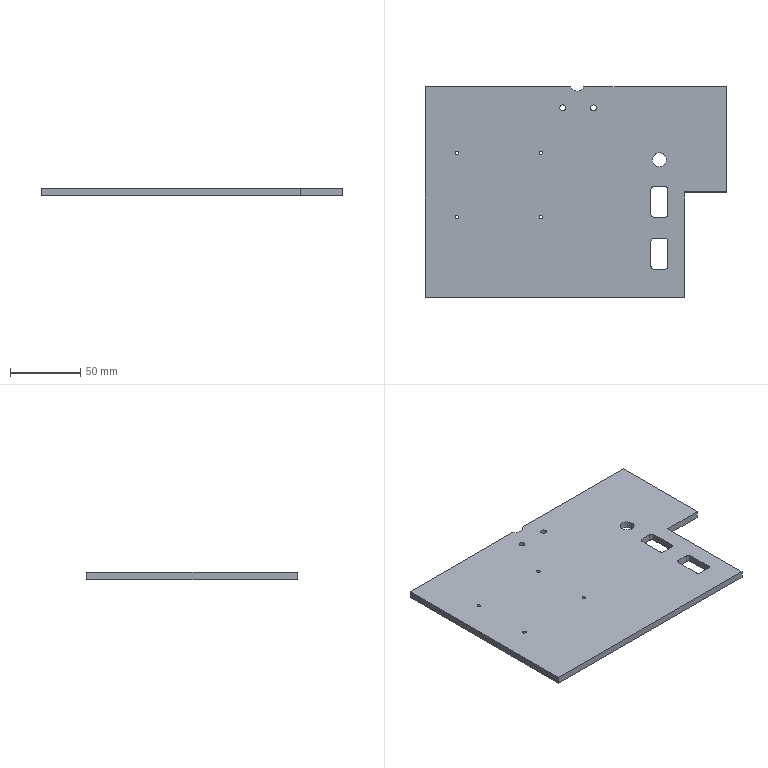Part | NX | features BREP 1 | 1 solid | 33 faces | box 215 x 150 x 5 mm | volume 146666 mm3 | plane 17 | cylinder 16 | commonest cylinder face diameters 4 x8 2.5 x4 4.2 x2 10 x2
STEP:
#1=CARTESIAN_POINT('',(-68.75,28.,0.));
#2=VERTEX_POINT('',#1);
#3=CARTESIAN_POINT('',(-70.,28.,0.));
#4=DIRECTION('',(0.,0.,1.));
#5=DIRECTION('',(1.,0.,0.));
#6=AXIS2_PLACEMENT_3D('',#3,#4,#5);
#7=CIRCLE('',#6,1.25);
#8=EDGE_CURVE('',#2,#2,#7,.T.);
#9=ORIENTED_EDGE('',*,*,#8,.T.);
#10=EDGE_LOOP('',(#9));
#11=FACE_BOUND('',#10,.T.);
#12=CARTESIAN_POINT('',(-71.25,28.,-5.));
#13=VERTEX_POINT('',#12);
#14=CARTESIAN_POINT('',(-70.,28.,-5.));
#15=DIRECTION('',(0.,0.,-1.));
#16=DIRECTION('',(-1.,0.,0.));
#17=AXIS2_PLACEMENT_3D('',#14,#15,#16);
#18=CIRCLE('',#17,1.25);
#19=EDGE_CURVE('',#13,#13,#18,.T.);
#20=ORIENTED_EDGE('',*,*,#19,.T.);
#21=EDGE_LOOP('',(#20));
#22=FACE_BOUND('',#21,.T.);
#23=CARTESIAN_POINT('',(-70.,28.,-10.));
#24=DIRECTION('',(0.,0.,1.));
#25=DIRECTION('',(1.,0.,0.));
#26=AXIS2_PLACEMENT_3D('',#23,#24,#25);
#27=CYLINDRICAL_SURFACE('',#26,1.25);
#28=ADVANCED_FACE('',(#11,#22),#27,.F.);
#29=CARTESIAN_POINT('',(-8.75,-18.,0.));
#30=VERTEX_POINT('',#29);
#31=CARTESIAN_POINT('',(-10.,-18.,0.));
#32=DIRECTION('',(0.,0.,1.));
#33=DIRECTION('',(1.,0.,0.));
#34=AXIS2_PLACEMENT_3D('',#31,#32,#33);
#35=CIRCLE('',#34,1.25);
#36=EDGE_CURVE('',#30,#30,#35,.T.);
#37=ORIENTED_EDGE('',*,*,#36,.T.);
#38=EDGE_LOOP('',(#37));
#39=FACE_BOUND('',#38,.T.);
#40=CARTESIAN_POINT('',(-11.25,-18.,-5.));
#41=VERTEX_POINT('',#40);
#42=CARTESIAN_POINT('',(-10.,-18.,-5.));
#43=DIRECTION('',(0.,0.,-1.));
#44=DIRECTION('',(-1.,0.,0.));
#45=AXIS2_PLACEMENT_3D('',#42,#43,#44);
#46=CIRCLE('',#45,1.25);
#47=EDGE_CURVE('',#41,#41,#46,.T.);
#48=ORIENTED_EDGE('',*,*,#47,.T.);
#49=EDGE_LOOP('',(#48));
#50=FACE_BOUND('',#49,.T.);
#51=CARTESIAN_POINT('',(-10.,-18.,-10.));
#52=DIRECTION('',(0.,0.,1.));
#53=DIRECTION('',(1.,0.,0.));
#54=AXIS2_PLACEMENT_3D('',#51,#52,#53);
#55=CYLINDRICAL_SURFACE('',#54,1.25);
#56=ADVANCED_FACE('',(#39,#50),#55,.F.);
#57=CARTESIAN_POINT('',(-8.75,28.,0.));
#58=VERTEX_POINT('',#57);
#59=CARTESIAN_POINT('',(-10.,28.,0.));
#60=DIRECTION('',(0.,0.,1.));
#61=DIRECTION('',(1.,0.,0.));
#62=AXIS2_PLACEMENT_3D('',#59,#60,#61);
#63=CIRCLE('',#62,1.25);
#64=EDGE_CURVE('',#58,#58,#63,.T.);
#65=ORIENTED_EDGE('',*,*,#64,.T.);
#66=EDGE_LOOP('',(#65));
#67=FACE_BOUND('',#66,.T.);
#68=CARTESIAN_POINT('',(-11.25,28.,-5.));
#69=VERTEX_POINT('',#68);
#70=CARTESIAN_POINT('',(-10.,28.,-5.));
#71=DIRECTION('',(0.,0.,-1.));
#72=DIRECTION('',(-1.,0.,0.));
#73=AXIS2_PLACEMENT_3D('',#70,#71,#72);
#74=CIRCLE('',#73,1.25);
#75=EDGE_CURVE('',#69,#69,#74,.T.);
#76=ORIENTED_EDGE('',*,*,#75,.T.);
#77=EDGE_LOOP('',(#76));
#78=FACE_BOUND('',#77,.T.);
#79=CARTESIAN_POINT('',(-10.,28.,-10.));
#80=DIRECTION('',(0.,0.,1.));
#81=DIRECTION('',(1.,0.,0.));
#82=AXIS2_PLACEMENT_3D('',#79,#80,#81);
#83=CYLINDRICAL_SURFACE('',#82,1.25);
#84=ADVANCED_FACE('',(#67,#78),#83,.F.);
#85=CARTESIAN_POINT('',(-68.75,-18.,0.));
#86=VERTEX_POINT('',#85);
#87=CARTESIAN_POINT('',(-70.,-18.,0.));
#88=DIRECTION('',(0.,0.,1.));
#89=DIRECTION('',(1.,0.,0.));
#90=AXIS2_PLACEMENT_3D('',#87,#88,#89);
#91=CIRCLE('',#90,1.25);
#92=EDGE_CURVE('',#86,#86,#91,.T.);
#93=ORIENTED_EDGE('',*,*,#92,.T.);
#94=EDGE_LOOP('',(#93));
#95=FACE_BOUND('',#94,.T.);
#96=CARTESIAN_POINT('',(-71.25,-18.,-5.));
#97=VERTEX_POINT('',#96);
#98=CARTESIAN_POINT('',(-70.,-18.,-5.));
#99=DIRECTION('',(0.,0.,-1.));
#100=DIRECTION('',(-1.,0.,0.));
#101=AXIS2_PLACEMENT_3D('',#98,#99,#100);
#102=CIRCLE('',#101,1.25);
#103=EDGE_CURVE('',#97,#97,#102,.T.);
#104=ORIENTED_EDGE('',*,*,#103,.T.);
#105=EDGE_LOOP('',(#104));
#106=FACE_BOUND('',#105,.T.);
#107=CARTESIAN_POINT('',(-70.,-18.,-10.));
#108=DIRECTION('',(0.,0.,1.));
#109=DIRECTION('',(1.,0.,0.));
#110=AXIS2_PLACEMENT_3D('',#107,#108,#109);
#111=CYLINDRICAL_SURFACE('',#110,1.25);
#112=ADVANCED_FACE('',(#95,#106),#111,.F.);
#113=CARTESIAN_POINT('',(3.4,60.,-5.));
#114=VERTEX_POINT('',#113);
#115=CARTESIAN_POINT('',(5.5,60.,-5.));
#116=DIRECTION('',(0.,0.,-1.));
#117=DIRECTION('',(-1.,0.,0.));
#118=AXIS2_PLACEMENT_3D('',#115,#116,#117);
#119=CIRCLE('',#118,2.1);
#120=EDGE_CURVE('',#114,#114,#119,.T.);
#121=ORIENTED_EDGE('',*,*,#120,.T.);
#122=EDGE_LOOP('',(#121));
#123=FACE_BOUND('',#122,.T.);
#124=CARTESIAN_POINT('',(3.4,60.,0.));
#125=VERTEX_POINT('',#124);
#126=CARTESIAN_POINT('',(5.5,60.,0.));
#127=DIRECTION('',(0.,0.,-1.));
#128=DIRECTION('',(-1.,0.,0.));
#129=AXIS2_PLACEMENT_3D('',#126,#127,#128);
#130=CIRCLE('',#129,2.1);
#131=EDGE_CURVE('',#125,#125,#130,.T.);
#132=ORIENTED_EDGE('',*,*,#131,.F.);
#133=EDGE_LOOP('',(#132));
#134=FACE_BOUND('',#133,.T.);
#135=CARTESIAN_POINT('',(5.5,60.,-5.));
#136=DIRECTION('',(0.,0.,-1.));
#137=DIRECTION('',(-1.,0.,0.));
#138=AXIS2_PLACEMENT_3D('',#135,#136,#137);
#139=CYLINDRICAL_SURFACE('',#138,2.1);
#140=ADVANCED_FACE('',(#123,#134),#139,.F.);
#141=CARTESIAN_POINT('',(25.4,60.,-5.));
#142=VERTEX_POINT('',#141);
#143=CARTESIAN_POINT('',(27.5,60.,-5.));
#144=DIRECTION('',(0.,0.,-1.));
#145=DIRECTION('',(-1.,0.,0.));
#146=AXIS2_PLACEMENT_3D('',#143,#144,#145);
#147=CIRCLE('',#146,2.1);
#148=EDGE_CURVE('',#142,#142,#147,.T.);
#149=ORIENTED_EDGE('',*,*,#148,.T.);
#150=EDGE_LOOP('',(#149));
#151=FACE_BOUND('',#150,.T.);
#152=CARTESIAN_POINT('',(25.4,60.,0.));
#153=VERTEX_POINT('',#152);
#154=CARTESIAN_POINT('',(27.5,60.,0.));
#155=DIRECTION('',(0.,0.,-1.));
#156=DIRECTION('',(-1.,0.,0.));
#157=AXIS2_PLACEMENT_3D('',#154,#155,#156);
#158=CIRCLE('',#157,2.1);
#159=EDGE_CURVE('',#153,#153,#158,.T.);
#160=ORIENTED_EDGE('',*,*,#159,.F.);
#161=EDGE_LOOP('',(#160));
#162=FACE_BOUND('',#161,.T.);
#163=CARTESIAN_POINT('',(27.5,60.,-5.));
#164=DIRECTION('',(0.,0.,-1.));
#165=DIRECTION('',(-1.,0.,0.));
#166=AXIS2_PLACEMENT_3D('',#163,#164,#165);
#167=CYLINDRICAL_SURFACE('',#166,2.1);
#168=ADVANCED_FACE('',(#151,#162),#167,.F.);
#169=CARTESIAN_POINT('',(79.5,23.,0.));
#170=VERTEX_POINT('',#169);
#171=CARTESIAN_POINT('',(74.5,23.,0.));
#172=DIRECTION('',(0.,0.,1.));
#173=DIRECTION('',(1.,0.,0.));
#174=AXIS2_PLACEMENT_3D('',#171,#172,#173);
#175=CIRCLE('',#174,5.);
#176=EDGE_CURVE('',#170,#170,#175,.T.);
#177=ORIENTED_EDGE('',*,*,#176,.T.);
#178=EDGE_LOOP('',(#177));
#179=FACE_BOUND('',#178,.T.);
#180=CARTESIAN_POINT('',(69.5,23.,-5.));
#181=VERTEX_POINT('',#180);
#182=CARTESIAN_POINT('',(74.5,23.,-5.));
#183=DIRECTION('',(0.,0.,-1.));
#184=DIRECTION('',(-1.,0.,0.));
#185=AXIS2_PLACEMENT_3D('',#182,#183,#184);
#186=CIRCLE('',#185,5.);
#187=EDGE_CURVE('',#181,#181,#186,.T.);
#188=ORIENTED_EDGE('',*,*,#187,.T.);
#189=EDGE_LOOP('',(#188));
#190=FACE_BOUND('',#189,.T.);
#191=CARTESIAN_POINT('',(74.5,23.,-10.));
#192=DIRECTION('',(0.,0.,1.));
#193=DIRECTION('',(1.,0.,0.));
#194=AXIS2_PLACEMENT_3D('',#191,#192,#193);
#195=CYLINDRICAL_SURFACE('',#194,5.);
#196=ADVANCED_FACE('',(#179,#190),#195,.F.);
#197=CARTESIAN_POINT('',(122.5,75.,-5.));
#198=VERTEX_POINT('',#197);
#199=CARTESIAN_POINT('',(20.583,75.,-5.));
#200=VERTEX_POINT('',#199);
#201=CARTESIAN_POINT('',(-92.5,75.,-5.));
#202=DIRECTION('',(-1.,0.,0.));
#203=VECTOR('',#202,1000.);
#204=LINE('',#201,#203);
#205=EDGE_CURVE('',#198,#200,#204,.T.);
#206=ORIENTED_EDGE('',*,*,#205,.T.);
#207=CARTESIAN_POINT('',(20.583,75.,0.));
#208=VERTEX_POINT('',#207);
#209=CARTESIAN_POINT('',(20.583,75.,-5.));
#210=DIRECTION('',(0.,0.,1.));
#211=VECTOR('',#210,1000.);
#212=LINE('',#209,#211);
#213=EDGE_CURVE('',#200,#208,#212,.T.);
#214=ORIENTED_EDGE('',*,*,#213,.T.);
#215=CARTESIAN_POINT('',(122.5,75.,0.));
#216=VERTEX_POINT('',#215);
#217=CARTESIAN_POINT('',(-92.5,75.,0.));
#218=DIRECTION('',(-1.,0.,0.));
#219=VECTOR('',#218,1000.);
#220=LINE('',#217,#219);
#221=EDGE_CURVE('',#216,#208,#220,.T.);
#222=ORIENTED_EDGE('',*,*,#221,.F.);
#223=CARTESIAN_POINT('',(122.5,75.,-5.));
#224=DIRECTION('',(0.,0.,1.));
#225=VECTOR('',#224,1000.);
#226=LINE('',#223,#225);
#227=EDGE_CURVE('',#198,#216,#226,.T.);
#228=ORIENTED_EDGE('',*,*,#227,.F.);
#229=EDGE_LOOP('',(#206,#214,#222,#228));
#230=FACE_BOUND('',#229,.T.);
#231=CARTESIAN_POINT('',(-92.5,75.,-5.));
#232=DIRECTION('',(0.,1.,0.));
#233=DIRECTION('',(0.,0.,1.));
#234=AXIS2_PLACEMENT_3D('',#231,#232,#233);
#235=PLANE('',#234);
#236=ADVANCED_FACE('',(#230),#235,.T.);
#237=CARTESIAN_POINT('',(11.417,75.,0.));
#238=VERTEX_POINT('',#237);
#239=CARTESIAN_POINT('',(-92.5,75.,0.));
#240=VERTEX_POINT('',#239);
#241=CARTESIAN_POINT('',(-92.5,75.,0.));
#242=DIRECTION('',(-1.,0.,0.));
#243=VECTOR('',#242,1000.);
#244=LINE('',#241,#243);
#245=EDGE_CURVE('',#238,#240,#244,.T.);
#246=ORIENTED_EDGE('',*,*,#245,.F.);
#247=CARTESIAN_POINT('',(11.417,75.,-5.));
#248=VERTEX_POINT('',#247);
#249=CARTESIAN_POINT('',(11.417,75.,-5.));
#250=DIRECTION('',(0.,0.,1.));
#251=VECTOR('',#250,1000.);
#252=LINE('',#249,#251);
#253=EDGE_CURVE('',#248,#238,#252,.T.);
#254=ORIENTED_EDGE('',*,*,#253,.F.);
#255=CARTESIAN_POINT('',(-92.5,75.,-5.));
#256=VERTEX_POINT('',#255);
#257=CARTESIAN_POINT('',(-92.5,75.,-5.));
#258=DIRECTION('',(-1.,0.,0.));
#259=VECTOR('',#258,1000.);
#260=LINE('',#257,#259);
#261=EDGE_CURVE('',#248,#256,#260,.T.);
#262=ORIENTED_EDGE('',*,*,#261,.T.);
#263=CARTESIAN_POINT('',(-92.5,75.,-5.));
#264=DIRECTION('',(0.,0.,1.));
#265=VECTOR('',#264,1000.);
#266=LINE('',#263,#265);
#267=EDGE_CURVE('',#256,#240,#266,.T.);
#268=ORIENTED_EDGE('',*,*,#267,.T.);
#269=EDGE_LOOP('',(#246,#254,#262,#268));
#270=FACE_BOUND('',#269,.T.);
#271=CARTESIAN_POINT('',(-92.5,75.,-5.));
#272=DIRECTION('',(0.,1.,0.));
#273=DIRECTION('',(0.,0.,1.));
#274=AXIS2_PLACEMENT_3D('',#271,#272,#273);
#275=PLANE('',#274);
#276=ADVANCED_FACE('',(#270),#275,.T.);
#277=ORIENTED_EDGE('',*,*,#19,.F.);
#278=EDGE_LOOP('',(#277));
#279=FACE_BOUND('',#278,.T.);
#280=ORIENTED_EDGE('',*,*,#47,.F.);
#281=EDGE_LOOP('',(#280));
#282=FACE_BOUND('',#281,.T.);
#283=ORIENTED_EDGE('',*,*,#75,.F.);
#284=EDGE_LOOP('',(#283));
#285=FACE_BOUND('',#284,.T.);
#286=ORIENTED_EDGE('',*,*,#103,.F.);
#287=EDGE_LOOP('',(#286));
#288=FACE_BOUND('',#287,.T.);
#289=ORIENTED_EDGE('',*,*,#120,.F.);
#290=EDGE_LOOP('',(#289));
#291=FACE_BOUND('',#290,.T.);
#292=ORIENTED_EDGE('',*,*,#148,.F.);
#293=EDGE_LOOP('',(#292));
#294=FACE_BOUND('',#293,.T.);
#295=CARTESIAN_POINT('',(68.5,-53.,-5.));
#296=VERTEX_POINT('',#295);
#297=CARTESIAN_POINT('',(68.5,-35.,-5.));
#298=VERTEX_POINT('',#297);
#299=CARTESIAN_POINT('',(68.5,0.,-5.));
#300=DIRECTION('',(0.,1.,0.));
#301=VECTOR('',#300,1000.);
#302=LINE('',#299,#301);
#303=EDGE_CURVE('',#296,#298,#302,.T.);
#304=ORIENTED_EDGE('',*,*,#303,.F.);
#305=CARTESIAN_POINT('',(70.5,-55.,-5.));
#306=VERTEX_POINT('',#305);
#307=CARTESIAN_POINT('',(70.5,-53.,-5.));
#308=DIRECTION('',(0.,0.,1.));
#309=DIRECTION('',(-1.,0.,0.));
#310=AXIS2_PLACEMENT_3D('',#307,#308,#309);
#311=CIRCLE('',#310,2.);
#312=EDGE_CURVE('',#296,#306,#311,.T.);
#313=ORIENTED_EDGE('',*,*,#312,.T.);
#314=CARTESIAN_POINT('',(78.5,-55.,-5.));
#315=VERTEX_POINT('',#314);
#316=CARTESIAN_POINT('',(0.,-55.,-5.));
#317=DIRECTION('',(-1.,0.,0.));
#318=VECTOR('',#317,1000.);
#319=LINE('',#316,#318);
#320=EDGE_CURVE('',#315,#306,#319,.T.);
#321=ORIENTED_EDGE('',*,*,#320,.F.);
#322=CARTESIAN_POINT('',(80.5,-53.,-5.));
#323=VERTEX_POINT('',#322);
#324=CARTESIAN_POINT('',(78.5,-53.,-5.));
#325=DIRECTION('',(0.,0.,1.));
#326=DIRECTION('',(-1.,0.,0.));
#327=AXIS2_PLACEMENT_3D('',#324,#325,#326);
#328=CIRCLE('',#327,2.);
#329=EDGE_CURVE('',#315,#323,#328,.T.);
#330=ORIENTED_EDGE('',*,*,#329,.T.);
#331=CARTESIAN_POINT('',(80.5,-35.,-5.));
#332=VERTEX_POINT('',#331);
#333=CARTESIAN_POINT('',(80.5,0.,-5.));
#334=DIRECTION('',(0.,-1.,0.));
#335=VECTOR('',#334,1000.);
#336=LINE('',#333,#335);
#337=EDGE_CURVE('',#332,#323,#336,.T.);
#338=ORIENTED_EDGE('',*,*,#337,.F.);
#339=CARTESIAN_POINT('',(78.5,-33.,-5.));
#340=VERTEX_POINT('',#339);
#341=CARTESIAN_POINT('',(78.5,-35.,-5.));
#342=DIRECTION('',(0.,0.,1.));
#343=DIRECTION('',(-1.,0.,0.));
#344=AXIS2_PLACEMENT_3D('',#341,#342,#343);
#345=CIRCLE('',#344,2.);
#346=EDGE_CURVE('',#332,#340,#345,.T.);
#347=ORIENTED_EDGE('',*,*,#346,.T.);
#348=CARTESIAN_POINT('',(70.5,-33.,-5.));
#349=VERTEX_POINT('',#348);
#350=CARTESIAN_POINT('',(0.,-33.,-5.));
#351=DIRECTION('',(1.,0.,0.));
#352=VECTOR('',#351,1000.);
#353=LINE('',#350,#352);
#354=EDGE_CURVE('',#349,#340,#353,.T.);
#355=ORIENTED_EDGE('',*,*,#354,.F.);
#356=CARTESIAN_POINT('',(70.5,-35.,-5.));
#357=DIRECTION('',(0.,0.,1.));
#358=DIRECTION('',(-1.,0.,0.));
#359=AXIS2_PLACEMENT_3D('',#356,#357,#358);
#360=CIRCLE('',#359,2.);
#361=EDGE_CURVE('',#349,#298,#360,.T.);
#362=ORIENTED_EDGE('',*,*,#361,.T.);
#363=EDGE_LOOP('',(#304,#313,#321,#330,#338,#347,#355,#362));
#364=FACE_BOUND('',#363,.T.);
#365=CARTESIAN_POINT('',(68.5,-16.,-5.));
#366=VERTEX_POINT('',#365);
#367=CARTESIAN_POINT('',(68.5,2.,-5.));
#368=VERTEX_POINT('',#367);
#369=CARTESIAN_POINT('',(68.5,0.,-5.));
#370=DIRECTION('',(0.,1.,0.));
#371=VECTOR('',#370,1000.);
#372=LINE('',#369,#371);
#373=EDGE_CURVE('',#366,#368,#372,.T.);
#374=ORIENTED_EDGE('',*,*,#373,.F.);
#375=CARTESIAN_POINT('',(70.5,-18.,-5.));
#376=VERTEX_POINT('',#375);
#377=CARTESIAN_POINT('',(70.5,-16.,-5.));
#378=DIRECTION('',(0.,0.,1.));
#379=DIRECTION('',(-1.,0.,0.));
#380=AXIS2_PLACEMENT_3D('',#377,#378,#379);
#381=CIRCLE('',#380,2.);
#382=EDGE_CURVE('',#366,#376,#381,.T.);
#383=ORIENTED_EDGE('',*,*,#382,.T.);
#384=CARTESIAN_POINT('',(78.5,-18.,-5.));
#385=VERTEX_POINT('',#384);
#386=CARTESIAN_POINT('',(0.,-18.,-5.));
#387=DIRECTION('',(-1.,0.,0.));
#388=VECTOR('',#387,1000.);
#389=LINE('',#386,#388);
#390=EDGE_CURVE('',#385,#376,#389,.T.);
#391=ORIENTED_EDGE('',*,*,#390,.F.);
#392=CARTESIAN_POINT('',(80.5,-16.,-5.));
#393=VERTEX_POINT('',#392);
#394=CARTESIAN_POINT('',(78.5,-16.,-5.));
#395=DIRECTION('',(0.,0.,1.));
#396=DIRECTION('',(-1.,0.,0.));
#397=AXIS2_PLACEMENT_3D('',#394,#395,#396);
#398=CIRCLE('',#397,2.);
#399=EDGE_CURVE('',#385,#393,#398,.T.);
#400=ORIENTED_EDGE('',*,*,#399,.T.);
#401=CARTESIAN_POINT('',(80.5,2.,-5.));
#402=VERTEX_POINT('',#401);
#403=CARTESIAN_POINT('',(80.5,0.,-5.));
#404=DIRECTION('',(0.,-1.,0.));
#405=VECTOR('',#404,1000.);
#406=LINE('',#403,#405);
#407=EDGE_CURVE('',#402,#393,#406,.T.);
#408=ORIENTED_EDGE('',*,*,#407,.F.);
#409=CARTESIAN_POINT('',(78.5,4.,-5.));
#410=VERTEX_POINT('',#409);
#411=CARTESIAN_POINT('',(78.5,2.,-5.));
#412=DIRECTION('',(0.,0.,1.));
#413=DIRECTION('',(-1.,0.,0.));
#414=AXIS2_PLACEMENT_3D('',#411,#412,#413);
#415=CIRCLE('',#414,2.);
#416=EDGE_CURVE('',#402,#410,#415,.T.);
#417=ORIENTED_EDGE('',*,*,#416,.T.);
#418=CARTESIAN_POINT('',(70.5,4.,-5.));
#419=VERTEX_POINT('',#418);
#420=CARTESIAN_POINT('',(0.,4.,-5.));
#421=DIRECTION('',(1.,0.,0.));
#422=VECTOR('',#421,1000.);
#423=LINE('',#420,#422);
#424=EDGE_CURVE('',#419,#410,#423,.T.);
#425=ORIENTED_EDGE('',*,*,#424,.F.);
#426=CARTESIAN_POINT('',(70.5,2.,-5.));
#427=DIRECTION('',(0.,0.,1.));
#428=DIRECTION('',(-1.,0.,0.));
#429=AXIS2_PLACEMENT_3D('',#426,#427,#428);
#430=CIRCLE('',#429,2.);
#431=EDGE_CURVE('',#419,#368,#430,.T.);
#432=ORIENTED_EDGE('',*,*,#431,.T.);
#433=EDGE_LOOP('',(#374,#383,#391,#400,#408,#417,#425,#432));
#434=FACE_BOUND('',#433,.T.);
#435=ORIENTED_EDGE('',*,*,#187,.F.);
#436=EDGE_LOOP('',(#435));
#437=FACE_BOUND('',#436,.T.);
#438=ORIENTED_EDGE('',*,*,#261,.F.);
#439=CARTESIAN_POINT('',(16.,77.,-5.));
#440=DIRECTION('',(0.,0.,-1.));
#441=DIRECTION('',(-1.,0.,0.));
#442=AXIS2_PLACEMENT_3D('',#439,#440,#441);
#443=CIRCLE('',#442,5.);
#444=EDGE_CURVE('',#200,#248,#443,.T.);
#445=ORIENTED_EDGE('',*,*,#444,.F.);
#446=ORIENTED_EDGE('',*,*,#205,.F.);
#447=CARTESIAN_POINT('',(122.5,0.,-5.));
#448=VERTEX_POINT('',#447);
#449=CARTESIAN_POINT('',(122.5,75.,-5.));
#450=DIRECTION('',(0.,1.,0.));
#451=VECTOR('',#450,1000.);
#452=LINE('',#449,#451);
#453=EDGE_CURVE('',#448,#198,#452,.T.);
#454=ORIENTED_EDGE('',*,*,#453,.F.);
#455=CARTESIAN_POINT('',(92.5,0.,-5.));
#456=VERTEX_POINT('',#455);
#457=CARTESIAN_POINT('',(92.5,0.,-5.));
#458=DIRECTION('',(1.,0.,0.));
#459=VECTOR('',#458,1000.);
#460=LINE('',#457,#459);
#461=EDGE_CURVE('',#456,#448,#460,.T.);
#462=ORIENTED_EDGE('',*,*,#461,.F.);
#463=CARTESIAN_POINT('',(92.5,-75.,-5.));
#464=VERTEX_POINT('',#463);
#465=CARTESIAN_POINT('',(92.5,-75.,-5.));
#466=DIRECTION('',(0.,1.,0.));
#467=VECTOR('',#466,1000.);
#468=LINE('',#465,#467);
#469=EDGE_CURVE('',#464,#456,#468,.T.);
#470=ORIENTED_EDGE('',*,*,#469,.F.);
#471=CARTESIAN_POINT('',(-92.5,-75.,-5.));
#472=VERTEX_POINT('',#471);
#473=CARTESIAN_POINT('',(-92.5,-75.,-5.));
#474=DIRECTION('',(1.,0.,0.));
#475=VECTOR('',#474,1000.);
#476=LINE('',#473,#475);
#477=EDGE_CURVE('',#472,#464,#476,.T.);
#478=ORIENTED_EDGE('',*,*,#477,.F.);
#479=CARTESIAN_POINT('',(-92.5,-75.,-5.));
#480=DIRECTION('',(0.,-1.,0.));
#481=VECTOR('',#480,1000.);
#482=LINE('',#479,#481);
#483=EDGE_CURVE('',#256,#472,#482,.T.);
#484=ORIENTED_EDGE('',*,*,#483,.F.);
#485=EDGE_LOOP('',(#438,#445,#446,#454,#462,#470,#478,#484));
#486=FACE_BOUND('',#485,.T.);
#487=CARTESIAN_POINT('',(0.,0.,-5.));
#488=DIRECTION('',(0.,0.,-1.));
#489=DIRECTION('',(-1.,0.,0.));
#490=AXIS2_PLACEMENT_3D('',#487,#488,#489);
#491=PLANE('',#490);
#492=ADVANCED_FACE('',(#279,#282,#285,#288,#291,#294,#364,#434,#437,#486),#491,.T.);
#493=ORIENTED_EDGE('',*,*,#8,.F.);
#494=EDGE_LOOP('',(#493));
#495=FACE_BOUND('',#494,.T.);
#496=ORIENTED_EDGE('',*,*,#36,.F.);
#497=EDGE_LOOP('',(#496));
#498=FACE_BOUND('',#497,.T.);
#499=ORIENTED_EDGE('',*,*,#64,.F.);
#500=EDGE_LOOP('',(#499));
#501=FACE_BOUND('',#500,.T.);
#502=ORIENTED_EDGE('',*,*,#92,.F.);
#503=EDGE_LOOP('',(#502));
#504=FACE_BOUND('',#503,.T.);
#505=ORIENTED_EDGE('',*,*,#131,.T.);
#506=EDGE_LOOP('',(#505));
#507=FACE_BOUND('',#506,.T.);
#508=ORIENTED_EDGE('',*,*,#159,.T.);
#509=EDGE_LOOP('',(#508));
#510=FACE_BOUND('',#509,.T.);
#511=CARTESIAN_POINT('',(70.5,-55.,0.));
#512=VERTEX_POINT('',#511);
#513=CARTESIAN_POINT('',(78.5,-55.,0.));
#514=VERTEX_POINT('',#513);
#515=CARTESIAN_POINT('',(68.5,-55.,0.));
#516=DIRECTION('',(1.,0.,0.));
#517=VECTOR('',#516,1000.);
#518=LINE('',#515,#517);
#519=EDGE_CURVE('',#512,#514,#518,.T.);
#520=ORIENTED_EDGE('',*,*,#519,.F.);
#521=CARTESIAN_POINT('',(68.5,-53.,0.));
#522=VERTEX_POINT('',#521);
#523=CARTESIAN_POINT('',(70.5,-53.,0.));
#524=DIRECTION('',(0.,0.,-1.));
#525=DIRECTION('',(-1.,0.,0.));
#526=AXIS2_PLACEMENT_3D('',#523,#524,#525);
#527=CIRCLE('',#526,2.);
#528=EDGE_CURVE('',#512,#522,#527,.T.);
#529=ORIENTED_EDGE('',*,*,#528,.T.);
#530=CARTESIAN_POINT('',(68.5,-35.,0.));
#531=VERTEX_POINT('',#530);
#532=CARTESIAN_POINT('',(68.5,-33.,0.));
#533=DIRECTION('',(0.,-1.,0.));
#534=VECTOR('',#533,1000.);
#535=LINE('',#532,#534);
#536=EDGE_CURVE('',#531,#522,#535,.T.);
#537=ORIENTED_EDGE('',*,*,#536,.F.);
#538=CARTESIAN_POINT('',(70.5,-33.,0.));
#539=VERTEX_POINT('',#538);
#540=CARTESIAN_POINT('',(70.5,-35.,0.));
#541=DIRECTION('',(0.,0.,-1.));
#542=DIRECTION('',(-1.,0.,0.));
#543=AXIS2_PLACEMENT_3D('',#540,#541,#542);
#544=CIRCLE('',#543,2.);
#545=EDGE_CURVE('',#531,#539,#544,.T.);
#546=ORIENTED_EDGE('',*,*,#545,.T.);
#547=CARTESIAN_POINT('',(78.5,-33.,0.));
#548=VERTEX_POINT('',#547);
#549=CARTESIAN_POINT('',(68.5,-33.,0.));
#550=DIRECTION('',(-1.,0.,0.));
#551=VECTOR('',#550,1000.);
#552=LINE('',#549,#551);
#553=EDGE_CURVE('',#548,#539,#552,.T.);
#554=ORIENTED_EDGE('',*,*,#553,.F.);
#555=CARTESIAN_POINT('',(80.5,-35.,0.));
#556=VERTEX_POINT('',#555);
#557=CARTESIAN_POINT('',(78.5,-35.,0.));
#558=DIRECTION('',(0.,0.,-1.));
#559=DIRECTION('',(-1.,0.,0.));
#560=AXIS2_PLACEMENT_3D('',#557,#558,#559);
#561=CIRCLE('',#560,2.);
#562=EDGE_CURVE('',#548,#556,#561,.T.);
#563=ORIENTED_EDGE('',*,*,#562,.T.);
#564=CARTESIAN_POINT('',(80.5,-53.,0.));
#565=VERTEX_POINT('',#564);
#566=CARTESIAN_POINT('',(80.5,-33.,0.));
#567=DIRECTION('',(0.,1.,0.));
#568=VECTOR('',#567,1000.);
#569=LINE('',#566,#568);
#570=EDGE_CURVE('',#565,#556,#569,.T.);
#571=ORIENTED_EDGE('',*,*,#570,.F.);
#572=CARTESIAN_POINT('',(78.5,-53.,0.));
#573=DIRECTION('',(0.,0.,-1.));
#574=DIRECTION('',(-1.,0.,0.));
#575=AXIS2_PLACEMENT_3D('',#572,#573,#574);
#576=CIRCLE('',#575,2.);
#577=EDGE_CURVE('',#565,#514,#576,.T.);
#578=ORIENTED_EDGE('',*,*,#577,.T.);
#579=EDGE_LOOP('',(#520,#529,#537,#546,#554,#563,#571,#578));
#580=FACE_BOUND('',#579,.T.);
#581=CARTESIAN_POINT('',(70.5,-18.,0.));
#582=VERTEX_POINT('',#581);
#583=CARTESIAN_POINT('',(78.5,-18.,0.));
#584=VERTEX_POINT('',#583);
#585=CARTESIAN_POINT('',(68.5,-18.,0.));
#586=DIRECTION('',(1.,0.,0.));
#587=VECTOR('',#586,1000.);
#588=LINE('',#585,#587);
#589=EDGE_CURVE('',#582,#584,#588,.T.);
#590=ORIENTED_EDGE('',*,*,#589,.F.);
#591=CARTESIAN_POINT('',(68.5,-16.,0.));
#592=VERTEX_POINT('',#591);
#593=CARTESIAN_POINT('',(70.5,-16.,0.));
#594=DIRECTION('',(0.,0.,-1.));
#595=DIRECTION('',(-1.,0.,0.));
#596=AXIS2_PLACEMENT_3D('',#593,#594,#595);
#597=CIRCLE('',#596,2.);
#598=EDGE_CURVE('',#582,#592,#597,.T.);
#599=ORIENTED_EDGE('',*,*,#598,.T.);
#600=CARTESIAN_POINT('',(68.5,2.,0.));
#601=VERTEX_POINT('',#600);
#602=CARTESIAN_POINT('',(68.5,4.,0.));
#603=DIRECTION('',(0.,-1.,0.));
#604=VECTOR('',#603,1000.);
#605=LINE('',#602,#604);
#606=EDGE_CURVE('',#601,#592,#605,.T.);
#607=ORIENTED_EDGE('',*,*,#606,.F.);
#608=CARTESIAN_POINT('',(70.5,4.,0.));
#609=VERTEX_POINT('',#608);
#610=CARTESIAN_POINT('',(70.5,2.,0.));
#611=DIRECTION('',(0.,0.,-1.));
#612=DIRECTION('',(-1.,0.,0.));
#613=AXIS2_PLACEMENT_3D('',#610,#611,#612);
#614=CIRCLE('',#613,2.);
#615=EDGE_CURVE('',#601,#609,#614,.T.);
#616=ORIENTED_EDGE('',*,*,#615,.T.);
#617=CARTESIAN_POINT('',(78.5,4.,0.));
#618=VERTEX_POINT('',#617);
#619=CARTESIAN_POINT('',(68.5,4.,0.));
#620=DIRECTION('',(-1.,0.,0.));
#621=VECTOR('',#620,1000.);
#622=LINE('',#619,#621);
#623=EDGE_CURVE('',#618,#609,#622,.T.);
#624=ORIENTED_EDGE('',*,*,#623,.F.);
#625=CARTESIAN_POINT('',(80.5,2.,0.));
#626=VERTEX_POINT('',#625);
#627=CARTESIAN_POINT('',(78.5,2.,0.));
#628=DIRECTION('',(0.,0.,-1.));
#629=DIRECTION('',(-1.,0.,0.));
#630=AXIS2_PLACEMENT_3D('',#627,#628,#629);
#631=CIRCLE('',#630,2.);
#632=EDGE_CURVE('',#618,#626,#631,.T.);
#633=ORIENTED_EDGE('',*,*,#632,.T.);
#634=CARTESIAN_POINT('',(80.5,-16.,0.));
#635=VERTEX_POINT('',#634);
#636=CARTESIAN_POINT('',(80.5,4.,0.));
#637=DIRECTION('',(0.,1.,0.));
#638=VECTOR('',#637,1000.);
#639=LINE('',#636,#638);
#640=EDGE_CURVE('',#635,#626,#639,.T.);
#641=ORIENTED_EDGE('',*,*,#640,.F.);
#642=CARTESIAN_POINT('',(78.5,-16.,0.));
#643=DIRECTION('',(0.,0.,-1.));
#644=DIRECTION('',(-1.,0.,0.));
#645=AXIS2_PLACEMENT_3D('',#642,#643,#644);
#646=CIRCLE('',#645,2.);
#647=EDGE_CURVE('',#635,#584,#646,.T.);
#648=ORIENTED_EDGE('',*,*,#647,.T.);
#649=EDGE_LOOP('',(#590,#599,#607,#616,#624,#633,#641,#648));
#650=FACE_BOUND('',#649,.T.);
#651=ORIENTED_EDGE('',*,*,#176,.F.);
#652=EDGE_LOOP('',(#651));
#653=FACE_BOUND('',#652,.T.);
#654=CARTESIAN_POINT('',(16.,77.,0.));
#655=DIRECTION('',(0.,0.,-1.));
#656=DIRECTION('',(-1.,0.,0.));
#657=AXIS2_PLACEMENT_3D('',#654,#655,#656);
#658=CIRCLE('',#657,5.);
#659=EDGE_CURVE('',#208,#238,#658,.T.);
#660=ORIENTED_EDGE('',*,*,#659,.T.);
#661=ORIENTED_EDGE('',*,*,#245,.T.);
#662=CARTESIAN_POINT('',(-92.5,-75.,0.));
#663=VERTEX_POINT('',#662);
#664=CARTESIAN_POINT('',(-92.5,-75.,0.));
#665=DIRECTION('',(0.,-1.,0.));
#666=VECTOR('',#665,1000.);
#667=LINE('',#664,#666);
#668=EDGE_CURVE('',#240,#663,#667,.T.);
#669=ORIENTED_EDGE('',*,*,#668,.T.);
#670=CARTESIAN_POINT('',(92.5,-75.,0.));
#671=VERTEX_POINT('',#670);
#672=CARTESIAN_POINT('',(-92.5,-75.,0.));
#673=DIRECTION('',(1.,0.,0.));
#674=VECTOR('',#673,1000.);
#675=LINE('',#672,#674);
#676=EDGE_CURVE('',#663,#671,#675,.T.);
#677=ORIENTED_EDGE('',*,*,#676,.T.);
#678=CARTESIAN_POINT('',(92.5,0.,0.));
#679=VERTEX_POINT('',#678);
#680=CARTESIAN_POINT('',(92.5,-75.,0.));
#681=DIRECTION('',(0.,1.,0.));
#682=VECTOR('',#681,1000.);
#683=LINE('',#680,#682);
#684=EDGE_CURVE('',#671,#679,#683,.T.);
#685=ORIENTED_EDGE('',*,*,#684,.T.);
#686=CARTESIAN_POINT('',(122.5,0.,0.));
#687=VERTEX_POINT('',#686);
#688=CARTESIAN_POINT('',(92.5,0.,0.));
#689=DIRECTION('',(1.,0.,0.));
#690=VECTOR('',#689,1000.);
#691=LINE('',#688,#690);
#692=EDGE_CURVE('',#679,#687,#691,.T.);
#693=ORIENTED_EDGE('',*,*,#692,.T.);
#694=CARTESIAN_POINT('',(122.5,75.,0.));
#695=DIRECTION('',(0.,1.,0.));
#696=VECTOR('',#695,1000.);
#697=LINE('',#694,#696);
#698=EDGE_CURVE('',#687,#216,#697,.T.);
#699=ORIENTED_EDGE('',*,*,#698,.T.);
#700=ORIENTED_EDGE('',*,*,#221,.T.);
#701=EDGE_LOOP('',(#660,#661,#669,#677,#685,#693,#699,#700));
#702=FACE_BOUND('',#701,.T.);
#703=CARTESIAN_POINT('',(0.,0.,0.));
#704=DIRECTION('',(0.,0.,-1.));
#705=DIRECTION('',(-1.,0.,0.));
#706=AXIS2_PLACEMENT_3D('',#703,#704,#705);
#707=PLANE('',#706);
#708=ADVANCED_FACE('',(#495,#498,#501,#504,#507,#510,#580,#650,#653,#702),#707,.F.);
#709=ORIENTED_EDGE('',*,*,#469,.T.);
#710=CARTESIAN_POINT('',(92.5,0.,-5.));
#711=DIRECTION('',(0.,0.,1.));
#712=VECTOR('',#711,1000.);
#713=LINE('',#710,#712);
#714=EDGE_CURVE('',#456,#679,#713,.T.);
#715=ORIENTED_EDGE('',*,*,#714,.T.);
#716=ORIENTED_EDGE('',*,*,#684,.F.);
#717=CARTESIAN_POINT('',(92.5,-75.,-5.));
#718=DIRECTION('',(0.,0.,1.));
#719=VECTOR('',#718,1000.);
#720=LINE('',#717,#719);
#721=EDGE_CURVE('',#464,#671,#720,.T.);
#722=ORIENTED_EDGE('',*,*,#721,.F.);
#723=EDGE_LOOP('',(#709,#715,#716,#722));
#724=FACE_BOUND('',#723,.T.);
#725=CARTESIAN_POINT('',(92.5,-75.,-5.));
#726=DIRECTION('',(1.,0.,0.));
#727=DIRECTION('',(0.,0.,-1.));
#728=AXIS2_PLACEMENT_3D('',#725,#726,#727);
#729=PLANE('',#728);
#730=ADVANCED_FACE('',(#724),#729,.T.);
#731=ORIENTED_EDGE('',*,*,#676,.F.);
#732=CARTESIAN_POINT('',(-92.5,-75.,-5.));
#733=DIRECTION('',(0.,0.,1.));
#734=VECTOR('',#733,1000.);
#735=LINE('',#732,#734);
#736=EDGE_CURVE('',#472,#663,#735,.T.);
#737=ORIENTED_EDGE('',*,*,#736,.F.);
#738=ORIENTED_EDGE('',*,*,#477,.T.);
#739=ORIENTED_EDGE('',*,*,#721,.T.);
#740=EDGE_LOOP('',(#731,#737,#738,#739));
#741=FACE_BOUND('',#740,.T.);
#742=CARTESIAN_POINT('',(-92.5,-75.,-5.));
#743=DIRECTION('',(0.,-1.,0.));
#744=DIRECTION('',(0.,0.,-1.));
#745=AXIS2_PLACEMENT_3D('',#742,#743,#744);
#746=PLANE('',#745);
#747=ADVANCED_FACE('',(#741),#746,.T.);
#748=ORIENTED_EDGE('',*,*,#668,.F.);
#749=ORIENTED_EDGE('',*,*,#267,.F.);
#750=ORIENTED_EDGE('',*,*,#483,.T.);
#751=ORIENTED_EDGE('',*,*,#736,.T.);
#752=EDGE_LOOP('',(#748,#749,#750,#751));
#753=FACE_BOUND('',#752,.T.);
#754=CARTESIAN_POINT('',(-92.5,-75.,-5.));
#755=DIRECTION('',(-1.,0.,0.));
#756=DIRECTION('',(0.,0.,1.));
#757=AXIS2_PLACEMENT_3D('',#754,#755,#756);
#758=PLANE('',#757);
#759=ADVANCED_FACE('',(#753),#758,.T.);
#760=ORIENTED_EDGE('',*,*,#698,.F.);
#761=CARTESIAN_POINT('',(122.5,0.,-5.));
#762=DIRECTION('',(0.,0.,1.));
#763=VECTOR('',#762,1000.);
#764=LINE('',#761,#763);
#765=EDGE_CURVE('',#448,#687,#764,.T.);
#766=ORIENTED_EDGE('',*,*,#765,.F.);
#767=ORIENTED_EDGE('',*,*,#453,.T.);
#768=ORIENTED_EDGE('',*,*,#227,.T.);
#769=EDGE_LOOP('',(#760,#766,#767,#768));
#770=FACE_BOUND('',#769,.T.);
#771=CARTESIAN_POINT('',(122.5,75.,-5.));
#772=DIRECTION('',(1.,0.,0.));
#773=DIRECTION('',(0.,1.,0.));
#774=AXIS2_PLACEMENT_3D('',#771,#772,#773);
#775=PLANE('',#774);
#776=ADVANCED_FACE('',(#770),#775,.T.);
#777=ORIENTED_EDGE('',*,*,#692,.F.);
#778=ORIENTED_EDGE('',*,*,#714,.F.);
#779=ORIENTED_EDGE('',*,*,#461,.T.);
#780=ORIENTED_EDGE('',*,*,#765,.T.);
#781=EDGE_LOOP('',(#777,#778,#779,#780));
#782=FACE_BOUND('',#781,.T.);
#783=CARTESIAN_POINT('',(92.5,0.,-5.));
#784=DIRECTION('',(0.,-1.,0.));
#785=DIRECTION('',(0.,0.,-1.));
#786=AXIS2_PLACEMENT_3D('',#783,#784,#785);
#787=PLANE('',#786);
#788=ADVANCED_FACE('',(#782),#787,.T.);
#789=ORIENTED_EDGE('',*,*,#444,.T.);
#790=ORIENTED_EDGE('',*,*,#253,.T.);
#791=ORIENTED_EDGE('',*,*,#659,.F.);
#792=ORIENTED_EDGE('',*,*,#213,.F.);
#793=EDGE_LOOP('',(#789,#790,#791,#792));
#794=FACE_BOUND('',#793,.T.);
#795=CARTESIAN_POINT('',(16.,77.,-5.));
#796=DIRECTION('',(0.,0.,-1.));
#797=DIRECTION('',(-1.,0.,0.));
#798=AXIS2_PLACEMENT_3D('',#795,#796,#797);
#799=CYLINDRICAL_SURFACE('',#798,5.);
#800=ADVANCED_FACE('',(#794),#799,.F.);
#801=ORIENTED_EDGE('',*,*,#373,.T.);
#802=CARTESIAN_POINT('',(68.5,2.,0.));
#803=DIRECTION('',(0.,0.,1.));
#804=VECTOR('',#803,1000.);
#805=LINE('',#802,#804);
#806=EDGE_CURVE('',#368,#601,#805,.T.);
#807=ORIENTED_EDGE('',*,*,#806,.T.);
#808=ORIENTED_EDGE('',*,*,#606,.T.);
#809=CARTESIAN_POINT('',(68.5,-16.,-5.));
#810=DIRECTION('',(0.,0.,-1.));
#811=VECTOR('',#810,1000.);
#812=LINE('',#809,#811);
#813=EDGE_CURVE('',#592,#366,#812,.T.);
#814=ORIENTED_EDGE('',*,*,#813,.T.);
#815=EDGE_LOOP('',(#801,#807,#808,#814));
#816=FACE_BOUND('',#815,.T.);
#817=CARTESIAN_POINT('',(68.5,4.,-10.));
#818=DIRECTION('',(-1.,0.,0.));
#819=DIRECTION('',(0.,0.,1.));
#820=AXIS2_PLACEMENT_3D('',#817,#818,#819);
#821=PLANE('',#820);
#822=ADVANCED_FACE('',(#816),#821,.F.);
#823=ORIENTED_EDGE('',*,*,#623,.T.);
#824=CARTESIAN_POINT('',(70.5,4.,-5.));
#825=DIRECTION('',(0.,0.,-1.));
#826=VECTOR('',#825,1000.);
#827=LINE('',#824,#826);
#828=EDGE_CURVE('',#609,#419,#827,.T.);
#829=ORIENTED_EDGE('',*,*,#828,.T.);
#830=ORIENTED_EDGE('',*,*,#424,.T.);
#831=CARTESIAN_POINT('',(78.5,4.,0.));
#832=DIRECTION('',(0.,0.,1.));
#833=VECTOR('',#832,1000.);
#834=LINE('',#831,#833);
#835=EDGE_CURVE('',#410,#618,#834,.T.);
#836=ORIENTED_EDGE('',*,*,#835,.T.);
#837=EDGE_LOOP('',(#823,#829,#830,#836));
#838=FACE_BOUND('',#837,.T.);
#839=CARTESIAN_POINT('',(68.5,4.,-10.));
#840=DIRECTION('',(0.,1.,0.));
#841=DIRECTION('',(0.,0.,1.));
#842=AXIS2_PLACEMENT_3D('',#839,#840,#841);
#843=PLANE('',#842);
#844=ADVANCED_FACE('',(#838),#843,.F.);
#845=ORIENTED_EDGE('',*,*,#640,.T.);
#846=CARTESIAN_POINT('',(80.5,2.,-5.));
#847=DIRECTION('',(0.,0.,-1.));
#848=VECTOR('',#847,1000.);
#849=LINE('',#846,#848);
#850=EDGE_CURVE('',#626,#402,#849,.T.);
#851=ORIENTED_EDGE('',*,*,#850,.T.);
#852=ORIENTED_EDGE('',*,*,#407,.T.);
#853=CARTESIAN_POINT('',(80.5,-16.,0.));
#854=DIRECTION('',(0.,0.,1.));
#855=VECTOR('',#854,1000.);
#856=LINE('',#853,#855);
#857=EDGE_CURVE('',#393,#635,#856,.T.);
#858=ORIENTED_EDGE('',*,*,#857,.T.);
#859=EDGE_LOOP('',(#845,#851,#852,#858));
#860=FACE_BOUND('',#859,.T.);
#861=CARTESIAN_POINT('',(80.5,4.,-10.));
#862=DIRECTION('',(1.,0.,0.));
#863=DIRECTION('',(0.,0.,-1.));
#864=AXIS2_PLACEMENT_3D('',#861,#862,#863);
#865=PLANE('',#864);
#866=ADVANCED_FACE('',(#860),#865,.F.);
#867=ORIENTED_EDGE('',*,*,#390,.T.);
#868=CARTESIAN_POINT('',(70.5,-18.,0.));
#869=DIRECTION('',(0.,0.,1.));
#870=VECTOR('',#869,1000.);
#871=LINE('',#868,#870);
#872=EDGE_CURVE('',#376,#582,#871,.T.);
#873=ORIENTED_EDGE('',*,*,#872,.T.);
#874=ORIENTED_EDGE('',*,*,#589,.T.);
#875=CARTESIAN_POINT('',(78.5,-18.,-5.));
#876=DIRECTION('',(0.,0.,-1.));
#877=VECTOR('',#876,1000.);
#878=LINE('',#875,#877);
#879=EDGE_CURVE('',#584,#385,#878,.T.);
#880=ORIENTED_EDGE('',*,*,#879,.T.);
#881=EDGE_LOOP('',(#867,#873,#874,#880));
#882=FACE_BOUND('',#881,.T.);
#883=CARTESIAN_POINT('',(68.5,-18.,-10.));
#884=DIRECTION('',(0.,-1.,0.));
#885=DIRECTION('',(0.,0.,-1.));
#886=AXIS2_PLACEMENT_3D('',#883,#884,#885);
#887=PLANE('',#886);
#888=ADVANCED_FACE('',(#882),#887,.F.);
#889=ORIENTED_EDGE('',*,*,#303,.T.);
#890=CARTESIAN_POINT('',(68.5,-35.,0.));
#891=DIRECTION('',(0.,0.,1.));
#892=VECTOR('',#891,1000.);
#893=LINE('',#890,#892);
#894=EDGE_CURVE('',#298,#531,#893,.T.);
#895=ORIENTED_EDGE('',*,*,#894,.T.);
#896=ORIENTED_EDGE('',*,*,#536,.T.);
#897=CARTESIAN_POINT('',(68.5,-53.,-5.));
#898=DIRECTION('',(0.,0.,-1.));
#899=VECTOR('',#898,1000.);
#900=LINE('',#897,#899);
#901=EDGE_CURVE('',#522,#296,#900,.T.);
#902=ORIENTED_EDGE('',*,*,#901,.T.);
#903=EDGE_LOOP('',(#889,#895,#896,#902));
#904=FACE_BOUND('',#903,.T.);
#905=CARTESIAN_POINT('',(68.5,-33.,-10.));
#906=DIRECTION('',(-1.,0.,0.));
#907=DIRECTION('',(0.,0.,1.));
#908=AXIS2_PLACEMENT_3D('',#905,#906,#907);
#909=PLANE('',#908);
#910=ADVANCED_FACE('',(#904),#909,.F.);
#911=ORIENTED_EDGE('',*,*,#553,.T.);
#912=CARTESIAN_POINT('',(70.5,-33.,-5.));
#913=DIRECTION('',(0.,0.,-1.));
#914=VECTOR('',#913,1000.);
#915=LINE('',#912,#914);
#916=EDGE_CURVE('',#539,#349,#915,.T.);
#917=ORIENTED_EDGE('',*,*,#916,.T.);
#918=ORIENTED_EDGE('',*,*,#354,.T.);
#919=CARTESIAN_POINT('',(78.5,-33.,0.));
#920=DIRECTION('',(0.,0.,1.));
#921=VECTOR('',#920,1000.);
#922=LINE('',#919,#921);
#923=EDGE_CURVE('',#340,#548,#922,.T.);
#924=ORIENTED_EDGE('',*,*,#923,.T.);
#925=EDGE_LOOP('',(#911,#917,#918,#924));
#926=FACE_BOUND('',#925,.T.);
#927=CARTESIAN_POINT('',(68.5,-33.,-10.));
#928=DIRECTION('',(0.,1.,0.));
#929=DIRECTION('',(0.,0.,1.));
#930=AXIS2_PLACEMENT_3D('',#927,#928,#929);
#931=PLANE('',#930);
#932=ADVANCED_FACE('',(#926),#931,.F.);
#933=ORIENTED_EDGE('',*,*,#570,.T.);
#934=CARTESIAN_POINT('',(80.5,-35.,-5.));
#935=DIRECTION('',(0.,0.,-1.));
#936=VECTOR('',#935,1000.);
#937=LINE('',#934,#936);
#938=EDGE_CURVE('',#556,#332,#937,.T.);
#939=ORIENTED_EDGE('',*,*,#938,.T.);
#940=ORIENTED_EDGE('',*,*,#337,.T.);
#941=CARTESIAN_POINT('',(80.5,-53.,0.));
#942=DIRECTION('',(0.,0.,1.));
#943=VECTOR('',#942,1000.);
#944=LINE('',#941,#943);
#945=EDGE_CURVE('',#323,#565,#944,.T.);
#946=ORIENTED_EDGE('',*,*,#945,.T.);
#947=EDGE_LOOP('',(#933,#939,#940,#946));
#948=FACE_BOUND('',#947,.T.);
#949=CARTESIAN_POINT('',(80.5,-33.,-10.));
#950=DIRECTION('',(1.,0.,0.));
#951=DIRECTION('',(0.,0.,-1.));
#952=AXIS2_PLACEMENT_3D('',#949,#950,#951);
#953=PLANE('',#952);
#954=ADVANCED_FACE('',(#948),#953,.F.);
#955=ORIENTED_EDGE('',*,*,#519,.T.);
#956=CARTESIAN_POINT('',(78.5,-55.,-5.));
#957=DIRECTION('',(0.,0.,-1.));
#958=VECTOR('',#957,1000.);
#959=LINE('',#956,#958);
#960=EDGE_CURVE('',#514,#315,#959,.T.);
#961=ORIENTED_EDGE('',*,*,#960,.T.);
#962=ORIENTED_EDGE('',*,*,#320,.T.);
#963=CARTESIAN_POINT('',(70.5,-55.,0.));
#964=DIRECTION('',(0.,0.,1.));
#965=VECTOR('',#964,1000.);
#966=LINE('',#963,#965);
#967=EDGE_CURVE('',#306,#512,#966,.T.);
#968=ORIENTED_EDGE('',*,*,#967,.T.);
#969=EDGE_LOOP('',(#955,#961,#962,#968));
#970=FACE_BOUND('',#969,.T.);
#971=CARTESIAN_POINT('',(68.5,-55.,-10.));
#972=DIRECTION('',(0.,-1.,0.));
#973=DIRECTION('',(0.,0.,-1.));
#974=AXIS2_PLACEMENT_3D('',#971,#972,#973);
#975=PLANE('',#974);
#976=ADVANCED_FACE('',(#970),#975,.F.);
#977=ORIENTED_EDGE('',*,*,#361,.F.);
#978=ORIENTED_EDGE('',*,*,#916,.F.);
#979=ORIENTED_EDGE('',*,*,#545,.F.);
#980=ORIENTED_EDGE('',*,*,#894,.F.);
#981=EDGE_LOOP('',(#977,#978,#979,#980));
#982=FACE_BOUND('',#981,.T.);
#983=CARTESIAN_POINT('',(70.5,-35.,-10.));
#984=DIRECTION('',(0.,0.,-1.));
#985=DIRECTION('',(-1.,0.,0.));
#986=AXIS2_PLACEMENT_3D('',#983,#984,#985);
#987=CYLINDRICAL_SURFACE('',#986,2.);
#988=ADVANCED_FACE('',(#982),#987,.F.);
#989=ORIENTED_EDGE('',*,*,#346,.F.);
#990=ORIENTED_EDGE('',*,*,#938,.F.);
#991=ORIENTED_EDGE('',*,*,#562,.F.);
#992=ORIENTED_EDGE('',*,*,#923,.F.);
#993=EDGE_LOOP('',(#989,#990,#991,#992));
#994=FACE_BOUND('',#993,.T.);
#995=CARTESIAN_POINT('',(78.5,-35.,-10.));
#996=DIRECTION('',(0.,0.,-1.));
#997=DIRECTION('',(-1.,0.,0.));
#998=AXIS2_PLACEMENT_3D('',#995,#996,#997);
#999=CYLINDRICAL_SURFACE('',#998,2.);
#1000=ADVANCED_FACE('',(#994),#999,.F.);
#1001=ORIENTED_EDGE('',*,*,#329,.F.);
#1002=ORIENTED_EDGE('',*,*,#960,.F.);
#1003=ORIENTED_EDGE('',*,*,#577,.F.);
#1004=ORIENTED_EDGE('',*,*,#945,.F.);
#1005=EDGE_LOOP('',(#1001,#1002,#1003,#1004));
#1006=FACE_BOUND('',#1005,.T.);
#1007=CARTESIAN_POINT('',(78.5,-53.,-10.));
#1008=DIRECTION('',(0.,0.,-1.));
#1009=DIRECTION('',(-1.,0.,0.));
#1010=AXIS2_PLACEMENT_3D('',#1007,#1008,#1009);
#1011=CYLINDRICAL_SURFACE('',#1010,2.);
#1012=ADVANCED_FACE('',(#1006),#1011,.F.);
#1013=ORIENTED_EDGE('',*,*,#312,.F.);
#1014=ORIENTED_EDGE('',*,*,#901,.F.);
#1015=ORIENTED_EDGE('',*,*,#528,.F.);
#1016=ORIENTED_EDGE('',*,*,#967,.F.);
#1017=EDGE_LOOP('',(#1013,#1014,#1015,#1016));
#1018=FACE_BOUND('',#1017,.T.);
#1019=CARTESIAN_POINT('',(70.5,-53.,-10.));
#1020=DIRECTION('',(0.,0.,-1.));
#1021=DIRECTION('',(-1.,0.,0.));
#1022=AXIS2_PLACEMENT_3D('',#1019,#1020,#1021);
#1023=CYLINDRICAL_SURFACE('',#1022,2.);
#1024=ADVANCED_FACE('',(#1018),#1023,.F.);
#1025=ORIENTED_EDGE('',*,*,#431,.F.);
#1026=ORIENTED_EDGE('',*,*,#828,.F.);
#1027=ORIENTED_EDGE('',*,*,#615,.F.);
#1028=ORIENTED_EDGE('',*,*,#806,.F.);
#1029=EDGE_LOOP('',(#1025,#1026,#1027,#1028));
#1030=FACE_BOUND('',#1029,.T.);
#1031=CARTESIAN_POINT('',(70.5,2.,-10.));
#1032=DIRECTION('',(0.,0.,-1.));
#1033=DIRECTION('',(-1.,0.,0.));
#1034=AXIS2_PLACEMENT_3D('',#1031,#1032,#1033);
#1035=CYLINDRICAL_SURFACE('',#1034,2.);
#1036=ADVANCED_FACE('',(#1030),#1035,.F.);
#1037=ORIENTED_EDGE('',*,*,#416,.F.);
#1038=ORIENTED_EDGE('',*,*,#850,.F.);
#1039=ORIENTED_EDGE('',*,*,#632,.F.);
#1040=ORIENTED_EDGE('',*,*,#835,.F.);
#1041=EDGE_LOOP('',(#1037,#1038,#1039,#1040));
#1042=FACE_BOUND('',#1041,.T.);
#1043=CARTESIAN_POINT('',(78.5,2.,-10.));
#1044=DIRECTION('',(0.,0.,-1.));
#1045=DIRECTION('',(-1.,0.,0.));
#1046=AXIS2_PLACEMENT_3D('',#1043,#1044,#1045);
#1047=CYLINDRICAL_SURFACE('',#1046,2.);
#1048=ADVANCED_FACE('',(#1042),#1047,.F.);
#1049=ORIENTED_EDGE('',*,*,#382,.F.);
#1050=ORIENTED_EDGE('',*,*,#813,.F.);
#1051=ORIENTED_EDGE('',*,*,#598,.F.);
#1052=ORIENTED_EDGE('',*,*,#872,.F.);
#1053=EDGE_LOOP('',(#1049,#1050,#1051,#1052));
#1054=FACE_BOUND('',#1053,.T.);
#1055=CARTESIAN_POINT('',(70.5,-16.,-10.));
#1056=DIRECTION('',(0.,0.,-1.));
#1057=DIRECTION('',(-1.,0.,0.));
#1058=AXIS2_PLACEMENT_3D('',#1055,#1056,#1057);
#1059=CYLINDRICAL_SURFACE('',#1058,2.);
#1060=ADVANCED_FACE('',(#1054),#1059,.F.);
#1061=ORIENTED_EDGE('',*,*,#399,.F.);
#1062=ORIENTED_EDGE('',*,*,#879,.F.);
#1063=ORIENTED_EDGE('',*,*,#647,.F.);
#1064=ORIENTED_EDGE('',*,*,#857,.F.);
#1065=EDGE_LOOP('',(#1061,#1062,#1063,#1064));
#1066=FACE_BOUND('',#1065,.T.);
#1067=CARTESIAN_POINT('',(78.5,-16.,-10.));
#1068=DIRECTION('',(0.,0.,-1.));
#1069=DIRECTION('',(-1.,0.,0.));
#1070=AXIS2_PLACEMENT_3D('',#1067,#1068,#1069);
#1071=CYLINDRICAL_SURFACE('',#1070,2.);
#1072=ADVANCED_FACE('',(#1066),#1071,.F.);
#1073=CLOSED_SHELL('',(#28,#56,#84,#112,#140,#168,#196,#236,#276,#492,#708,#730,#747,#759,#776,#788,#800,#822,#844,#866,#888,#910,#932,#954,#976,#988,#1000,#1012,#1024,#1036,#1048,#1060,#1072));
#1074=MANIFOLD_SOLID_BREP('',#1073);
#1075=(LENGTH_UNIT()NAMED_UNIT(*)SI_UNIT(.MILLI.,.METRE.));
#1076=UNCERTAINTY_MEASURE_WITH_UNIT(LENGTH_MEASURE(0.00001),#1075,'','');
#1077=(NAMED_UNIT(*)PLANE_ANGLE_UNIT()SI_UNIT($,.RADIAN.));
#1078=(NAMED_UNIT(*)SI_UNIT($,.STERADIAN.)SOLID_ANGLE_UNIT());
#1079=(GEOMETRIC_REPRESENTATION_CONTEXT(3)GLOBAL_UNCERTAINTY_ASSIGNED_CONTEXT((#1076))GLOBAL_UNIT_ASSIGNED_CONTEXT((#1075,#1077,#1078))REPRESENTATION_CONTEXT('',''));
#1080=ADVANCED_BREP_SHAPE_REPRESENTATION('',(#1074),#1079);